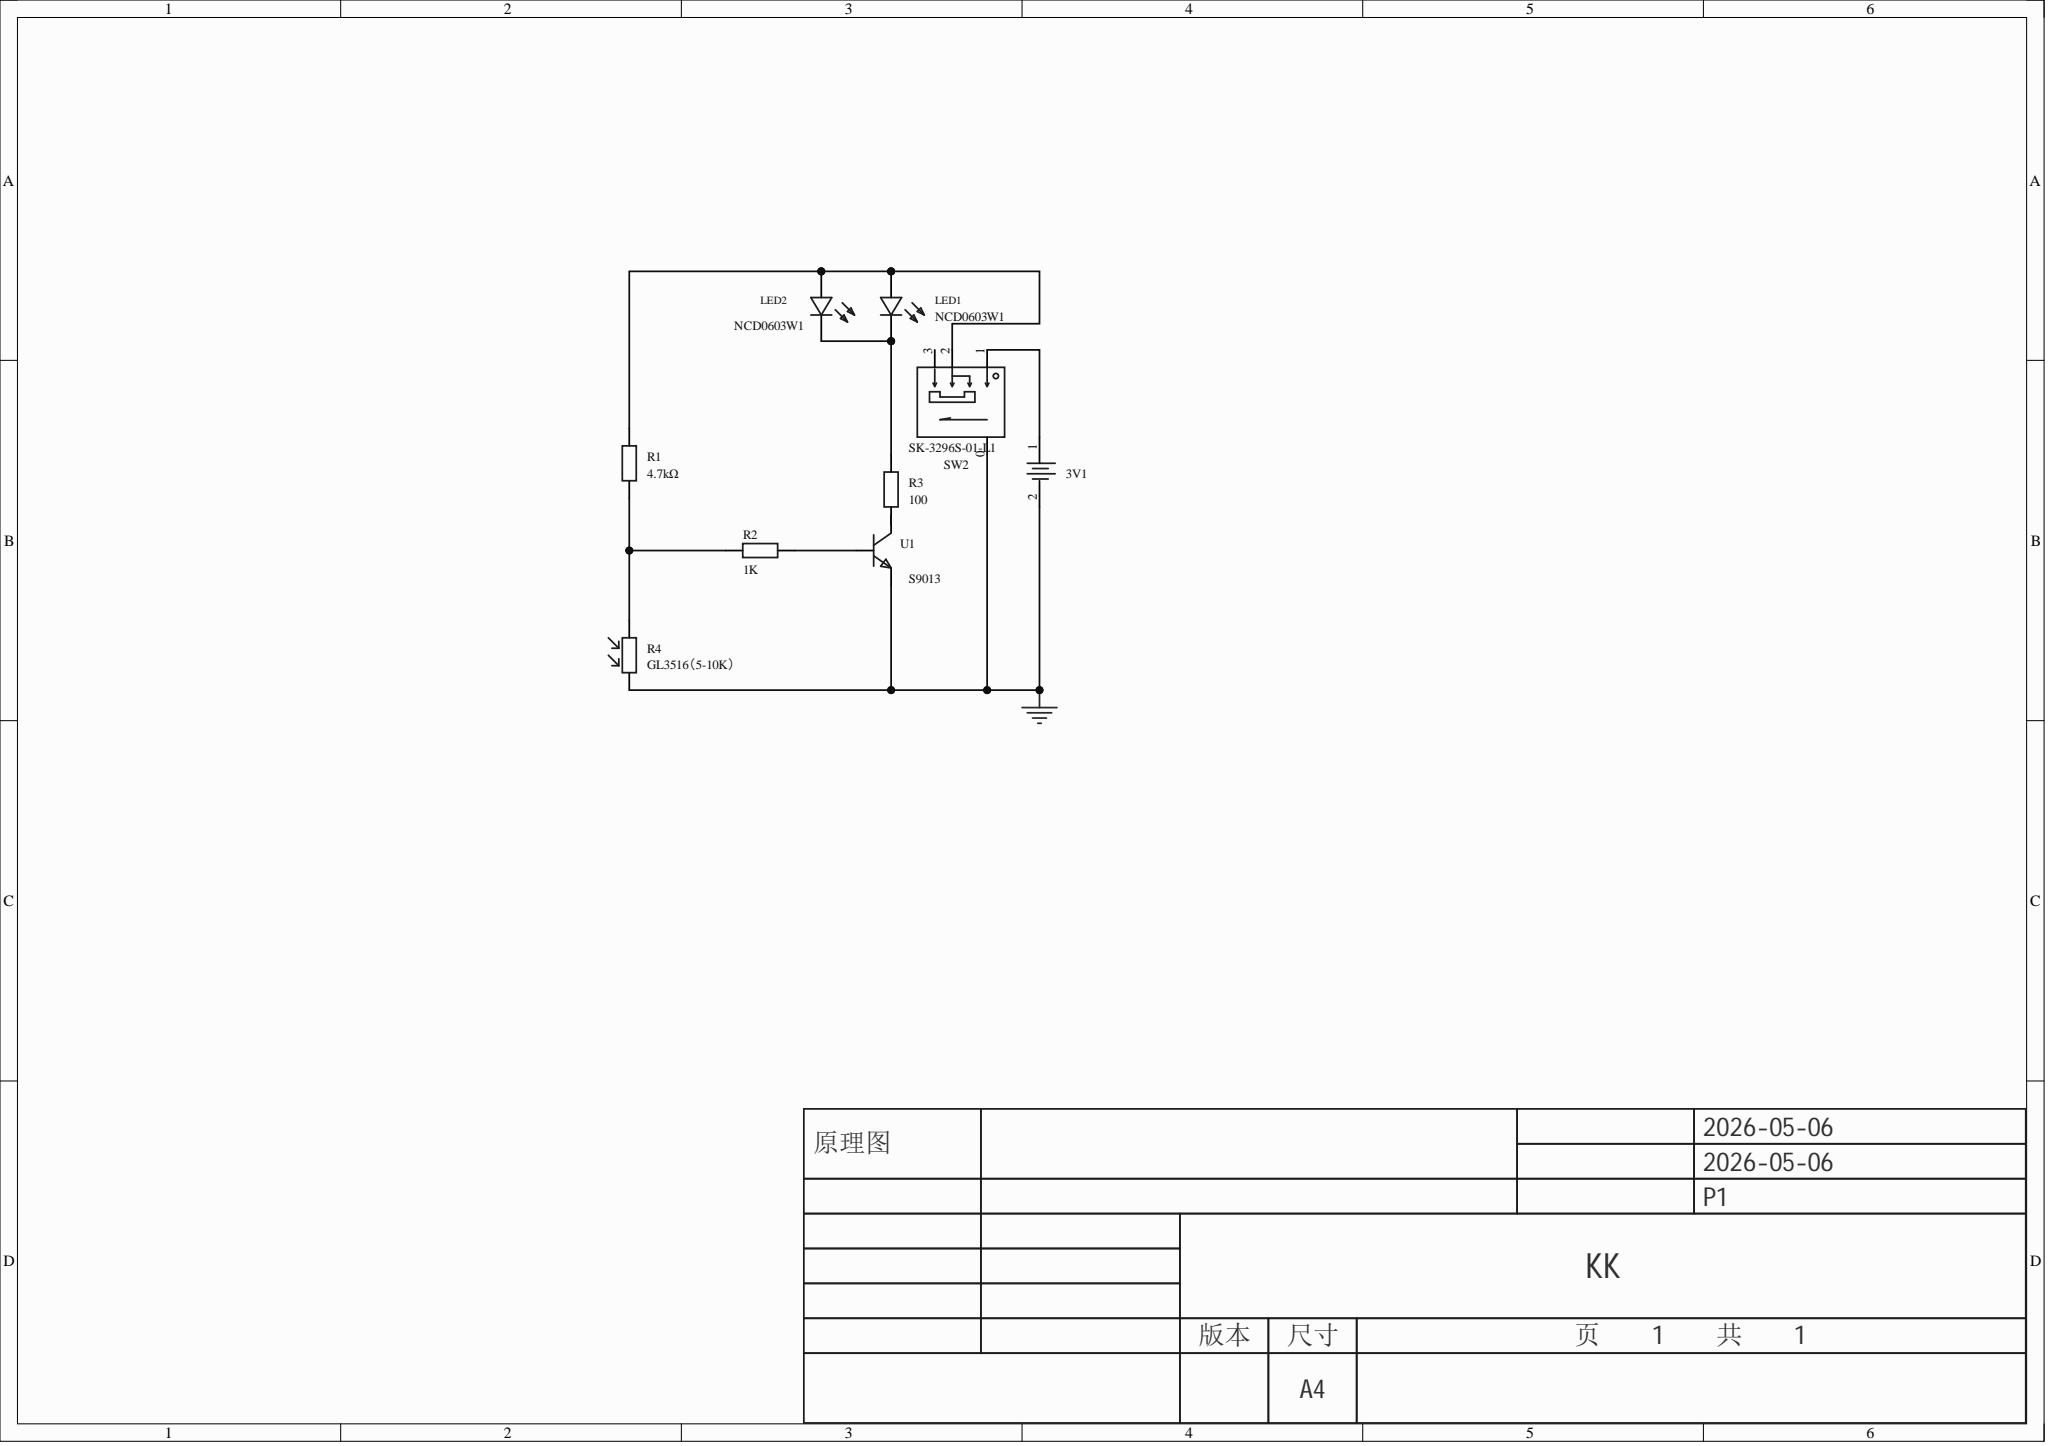Circuit board | Altium Designer | 9 parts | 7 nets
Bill of materials:
Comment,Description,Designator,Footprint,LibRef,Quantity
"","","3V1","BAT-TH_CR2032-BS-6-1","CR2032-BS-6-1 COPY","1"
"NCD0603W1","","LED1, LED2","LED0603-RD","NCD0603W1","2"
"4.7kΩ","","R1","R0805","0805W8F4701T5E","1"
"1K","","R2","R0805","0805W8F4701T5E","1"
"100","","R3","R0805","Res_0805","1"
"GL3516（5-10K）","","R4","RES-TH_L5.1-W4.3-P3.40-D0.5","GL3516（5-10K）","1"
"SK-3296S-01-L1","","SW2","SW-SMD_3P-P1.50_L2.7-W6.6","SK-3296S-01-L1","1"
"S9013","","U1","SOT-23-3_L2.9-W1.3-P1.90-LS2.4-BR","S9013_C5184425","1"
Netlist (Protel format):
[
3V1
BAT-TH_CR2032-BS-6-1




]
[
LED1
LED0603-RD
NCD0603W1



]
[
LED2
LED0603-RD
NCD0603W1



]
[
R1
R0805
4.7kΩ



]
[
R2
R0805
1K



]
[
R3
R0805
100



]
[
R4
RES-TH_L5.1-W4.3-P3.40-D0.5
GL3516（5-10K）



]
[
SW2
SW-SMD_3P-P1.50_L2.7-W6.6
SK-3296S-01-L1



]
[
U1
SOT-23-3_L2.9-W1.3-P1.90-LS2.4-BR
S9013



]
(
NetR3_1
R3-1
U1-3
)
(
NetR2_1
R2-1
U1-1
)
(
NetR1_1
R1-1
R2-2
R4-1
)
(
NetLED1_2
LED1-2
LED2-2
R1-2
SW2-2
)
(
NetLED1_1
LED1-1
LED2-1
R3-2
)
(
Net3V1_1
3V1-1
SW2-1
)
(
GND
3V1-2
R4-2
SW2-0
U1-2
)